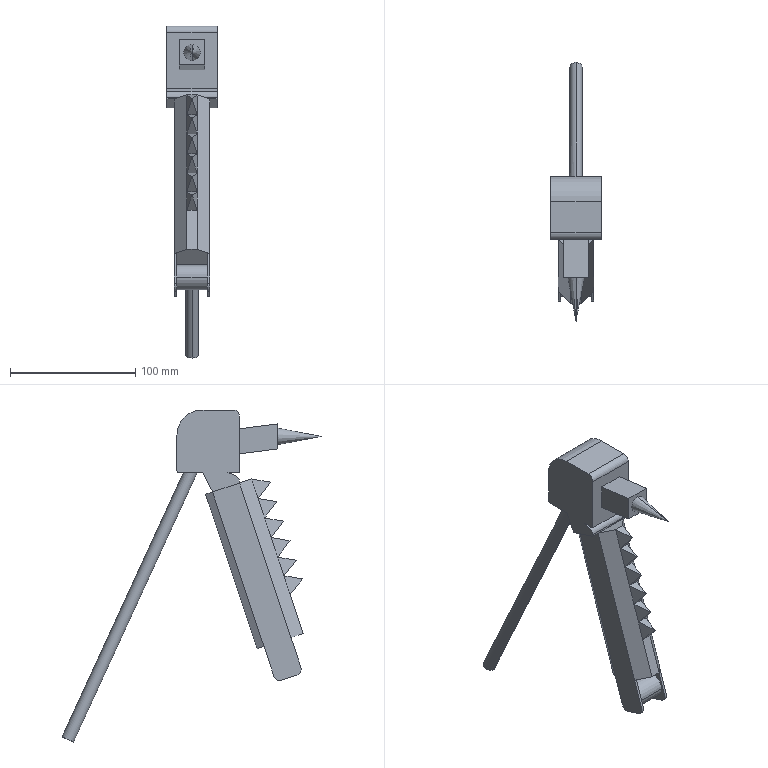Part | SolidWorks | features ICE 8, Fillet 5, Revolution 2, Extrusion 1 | 1 solid | 76 faces | box 40 x 207.302 x 265.068 mm | volume 279410 mm3 | plane 61 | cylinder 13 | cone 2 | commonest cylinder face diameters 10 x9 20 x2 4 x1 40 x1